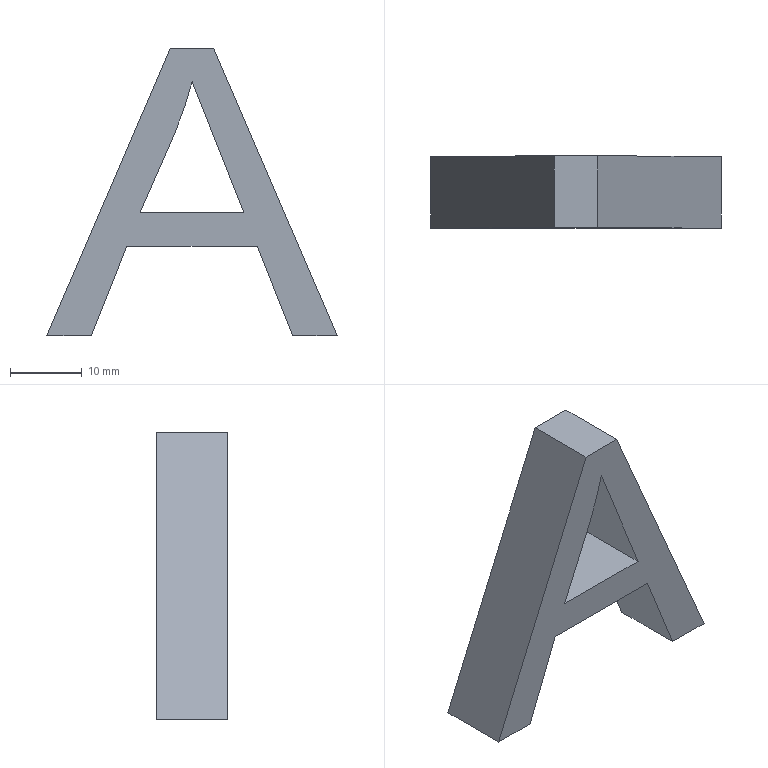Part | NX | features solid 2 | 1 solid | 14 faces | box 40.444 x 10 x 40 mm | volume 5154 mm3 | plane 12 | spline 2
STEP:
#1=CARTESIAN_POINT('',(-526.132,-915.,172.421));
#2=VERTEX_POINT('',#1);
#3=CARTESIAN_POINT('',(-533.352,-915.,190.669));
#4=VERTEX_POINT('',#3);
#5=CARTESIAN_POINT('',(-526.132,-915.,172.421));
#6=CARTESIAN_POINT('',(-527.509,-915.,175.908));
#7=CARTESIAN_POINT('',(-528.886,-915.,179.396));
#8=CARTESIAN_POINT('',(-531.586,-915.,186.236));
#9=CARTESIAN_POINT('',(-532.618,-915.,188.834));
#10=CARTESIAN_POINT('',(-533.352,-915.,190.669));
#11=B_SPLINE_CURVE_WITH_KNOTS('',3,(#5,#6,#7,#8,#9,#10),.UNSPECIFIED.,.F.,.F.,(4,2,4),(0.4694,0.6682,0.8594),.UNSPECIFIED.);
#12=EDGE_CURVE('',#2,#4,#11,.T.);
#13=ORIENTED_EDGE('',*,*,#12,.F.);
#14=CARTESIAN_POINT('',(-526.132,-925.,172.421));
#15=VERTEX_POINT('',#14);
#16=CARTESIAN_POINT('',(-526.132,-925.,172.421));
#17=DIRECTION('',(0.,1.,0.));
#18=VECTOR('',#17,1000.);
#19=LINE('',#16,#18);
#20=EDGE_CURVE('',#15,#2,#19,.T.);
#21=ORIENTED_EDGE('',*,*,#20,.F.);
#22=CARTESIAN_POINT('',(-533.352,-925.,190.669));
#23=VERTEX_POINT('',#22);
#24=CARTESIAN_POINT('',(-526.132,-925.,172.421));
#25=CARTESIAN_POINT('',(-527.509,-925.,175.908));
#26=CARTESIAN_POINT('',(-528.886,-925.,179.396));
#27=CARTESIAN_POINT('',(-531.586,-925.,186.236));
#28=CARTESIAN_POINT('',(-532.618,-925.,188.834));
#29=CARTESIAN_POINT('',(-533.352,-925.,190.669));
#30=B_SPLINE_CURVE_WITH_KNOTS('',3,(#24,#25,#26,#27,#28,#29),.UNSPECIFIED.,.F.,.F.,(4,2,4),(0.4694,0.6682,0.8594),.UNSPECIFIED.);
#31=EDGE_CURVE('',#15,#23,#30,.T.);
#32=ORIENTED_EDGE('',*,*,#31,.T.);
#33=CARTESIAN_POINT('',(-533.352,-925.,190.669));
#34=DIRECTION('',(0.,1.,0.));
#35=VECTOR('',#34,1000.);
#36=LINE('',#33,#35);
#37=EDGE_CURVE('',#23,#4,#36,.T.);
#38=ORIENTED_EDGE('',*,*,#37,.T.);
#39=EDGE_LOOP('',(#13,#21,#32,#38));
#40=FACE_BOUND('',#39,.T.);
#41=CARTESIAN_POINT('',(-526.132,-925.,172.421));
#42=CARTESIAN_POINT('',(-526.132,-915.,172.421));
#43=CARTESIAN_POINT('',(-526.807,-925.,174.131));
#44=CARTESIAN_POINT('',(-526.807,-915.,174.131));
#45=CARTESIAN_POINT('',(-527.821,-925.,176.699));
#46=CARTESIAN_POINT('',(-527.821,-915.,176.699));
#47=CARTESIAN_POINT('',(-529.168,-925.,180.111));
#48=CARTESIAN_POINT('',(-529.168,-915.,180.111));
#49=CARTESIAN_POINT('',(-530.19,-925.,182.699));
#50=CARTESIAN_POINT('',(-530.19,-915.,182.699));
#51=CARTESIAN_POINT('',(-531.169,-925.,185.178));
#52=CARTESIAN_POINT('',(-531.169,-915.,185.178));
#53=CARTESIAN_POINT('',(-532.298,-925.,188.027));
#54=CARTESIAN_POINT('',(-532.298,-915.,188.027));
#55=CARTESIAN_POINT('',(-532.978,-925.,189.733));
#56=CARTESIAN_POINT('',(-532.978,-915.,189.733));
#57=CARTESIAN_POINT('',(-533.352,-925.,190.669));
#58=CARTESIAN_POINT('',(-533.352,-915.,190.669));
#59=B_SPLINE_SURFACE_WITH_KNOTS('',3,1,((#41,#42),(#43,#44),(#45,#46),(#47,#48),(#49,#50),(#51,#52),(#53,#54),(#55,#56),(#57,#58)),.SURF_OF_LINEAR_EXTRUSION.,.F.,.F.,.F.,(4,1,1,1,1,1,4),(2,2),(0.4694,0.5669,0.6156,0.6644,0.7131,0.7619,0.8594),(0.,1.),.UNSPECIFIED.);
#60=ADVANCED_FACE('',(#40),#59,.T.);
#61=CARTESIAN_POINT('',(-535.754,-915.,183.511));
#62=VERTEX_POINT('',#61);
#63=CARTESIAN_POINT('',(-533.352,-915.,190.669));
#64=CARTESIAN_POINT('',(-533.918,-915.,188.39));
#65=CARTESIAN_POINT('',(-534.729,-915.,186.004));
#66=CARTESIAN_POINT('',(-535.754,-915.,183.511));
#67=B_SPLINE_CURVE_WITH_KNOTS('',3,(#63,#64,#65,#66),.UNSPECIFIED.,.F.,.F.,(4,4),(0.8594,1.),.PIECEWISE_BEZIER_KNOTS.);
#68=EDGE_CURVE('',#4,#62,#67,.T.);
#69=ORIENTED_EDGE('',*,*,#68,.F.);
#70=ORIENTED_EDGE('',*,*,#37,.F.);
#71=CARTESIAN_POINT('',(-535.754,-925.,183.511));
#72=VERTEX_POINT('',#71);
#73=CARTESIAN_POINT('',(-533.352,-925.,190.669));
#74=CARTESIAN_POINT('',(-533.918,-925.,188.39));
#75=CARTESIAN_POINT('',(-534.729,-925.,186.004));
#76=CARTESIAN_POINT('',(-535.754,-925.,183.511));
#77=B_SPLINE_CURVE_WITH_KNOTS('',3,(#73,#74,#75,#76),.UNSPECIFIED.,.F.,.F.,(4,4),(0.8594,1.),.PIECEWISE_BEZIER_KNOTS.);
#78=EDGE_CURVE('',#23,#72,#77,.T.);
#79=ORIENTED_EDGE('',*,*,#78,.T.);
#80=CARTESIAN_POINT('',(-535.754,-925.,183.511));
#81=DIRECTION('',(0.,1.,0.));
#82=VECTOR('',#81,1000.);
#83=LINE('',#80,#82);
#84=EDGE_CURVE('',#72,#62,#83,.T.);
#85=ORIENTED_EDGE('',*,*,#84,.T.);
#86=EDGE_LOOP('',(#69,#70,#79,#85));
#87=FACE_BOUND('',#86,.T.);
#88=CARTESIAN_POINT('',(-533.352,-925.,190.669));
#89=CARTESIAN_POINT('',(-533.352,-915.,190.669));
#90=CARTESIAN_POINT('',(-533.918,-925.,188.39));
#91=CARTESIAN_POINT('',(-533.918,-915.,188.39));
#92=CARTESIAN_POINT('',(-534.729,-925.,186.004));
#93=CARTESIAN_POINT('',(-534.729,-915.,186.004));
#94=CARTESIAN_POINT('',(-535.754,-925.,183.511));
#95=CARTESIAN_POINT('',(-535.754,-915.,183.511));
#96=B_SPLINE_SURFACE_WITH_KNOTS('',3,1,((#88,#89),(#90,#91),(#92,#93),(#94,#95)),.SURF_OF_LINEAR_EXTRUSION.,.F.,.F.,.F.,(4,4),(2,2),(0.8594,1.),(0.,1.),.PIECEWISE_BEZIER_KNOTS.);
#97=ADVANCED_FACE('',(#87),#96,.T.);
#98=CARTESIAN_POINT('',(-540.587,-915.,172.421));
#99=VERTEX_POINT('',#98);
#100=CARTESIAN_POINT('',(-535.754,-915.,183.511));
#101=CARTESIAN_POINT('',(-537.365,-915.,179.814));
#102=CARTESIAN_POINT('',(-538.976,-915.,176.117));
#103=CARTESIAN_POINT('',(-540.587,-915.,172.421));
#104=B_SPLINE_CURVE_WITH_KNOTS('',3,(#100,#101,#102,#103),.UNSPECIFIED.,.F.,.F.,(4,4),(0.,0.2138),.PIECEWISE_BEZIER_KNOTS.);
#105=EDGE_CURVE('',#62,#99,#104,.T.);
#106=ORIENTED_EDGE('',*,*,#105,.F.);
#107=ORIENTED_EDGE('',*,*,#84,.F.);
#108=CARTESIAN_POINT('',(-540.587,-925.,172.421));
#109=VERTEX_POINT('',#108);
#110=CARTESIAN_POINT('',(-535.754,-925.,183.511));
#111=CARTESIAN_POINT('',(-537.365,-925.,179.814));
#112=CARTESIAN_POINT('',(-538.976,-925.,176.117));
#113=CARTESIAN_POINT('',(-540.587,-925.,172.421));
#114=B_SPLINE_CURVE_WITH_KNOTS('',3,(#110,#111,#112,#113),.UNSPECIFIED.,.F.,.F.,(4,4),(0.,0.2138),.PIECEWISE_BEZIER_KNOTS.);
#115=EDGE_CURVE('',#72,#109,#114,.T.);
#116=ORIENTED_EDGE('',*,*,#115,.T.);
#117=CARTESIAN_POINT('',(-540.587,-925.,172.421));
#118=DIRECTION('',(0.,1.,0.));
#119=VECTOR('',#118,1000.);
#120=LINE('',#117,#119);
#121=EDGE_CURVE('',#109,#99,#120,.T.);
#122=ORIENTED_EDGE('',*,*,#121,.T.);
#123=EDGE_LOOP('',(#106,#107,#116,#122));
#124=FACE_BOUND('',#123,.T.);
#125=CARTESIAN_POINT('',(-535.754,-925.,183.511));
#126=DIRECTION('',(0.9167,0.,-0.3996));
#127=DIRECTION('',(0.3996,0.,0.9167));
#128=AXIS2_PLACEMENT_3D('',#125,#126,#127);
#129=PLANE('',#128);
#130=ADVANCED_FACE('',(#124),#129,.T.);
#131=CARTESIAN_POINT('',(-547.364,-915.,155.335));
#132=VERTEX_POINT('',#131);
#133=CARTESIAN_POINT('',(-553.574,-915.,155.335));
#134=VERTEX_POINT('',#133);
#135=CARTESIAN_POINT('',(-547.364,-915.,155.335));
#136=CARTESIAN_POINT('',(-549.434,-915.,155.335));
#137=CARTESIAN_POINT('',(-551.504,-915.,155.335));
#138=CARTESIAN_POINT('',(-553.574,-915.,155.335));
#139=B_SPLINE_CURVE_WITH_KNOTS('',3,(#135,#136,#137,#138),.UNSPECIFIED.,.F.,.F.,(4,4),(0.,0.04128),.PIECEWISE_BEZIER_KNOTS.);
#140=EDGE_CURVE('',#132,#134,#139,.T.);
#141=ORIENTED_EDGE('',*,*,#140,.F.);
#142=CARTESIAN_POINT('',(-547.364,-925.,155.335));
#143=VERTEX_POINT('',#142);
#144=CARTESIAN_POINT('',(-547.364,-925.,155.335));
#145=DIRECTION('',(0.,1.,0.));
#146=VECTOR('',#145,1000.);
#147=LINE('',#144,#146);
#148=EDGE_CURVE('',#143,#132,#147,.T.);
#149=ORIENTED_EDGE('',*,*,#148,.F.);
#150=CARTESIAN_POINT('',(-553.574,-925.,155.335));
#151=VERTEX_POINT('',#150);
#152=CARTESIAN_POINT('',(-547.364,-925.,155.335));
#153=CARTESIAN_POINT('',(-549.434,-925.,155.335));
#154=CARTESIAN_POINT('',(-551.504,-925.,155.335));
#155=CARTESIAN_POINT('',(-553.574,-925.,155.335));
#156=B_SPLINE_CURVE_WITH_KNOTS('',3,(#152,#153,#154,#155),.UNSPECIFIED.,.F.,.F.,(4,4),(0.,0.04128),.PIECEWISE_BEZIER_KNOTS.);
#157=EDGE_CURVE('',#143,#151,#156,.T.);
#158=ORIENTED_EDGE('',*,*,#157,.T.);
#159=CARTESIAN_POINT('',(-553.574,-925.,155.335));
#160=DIRECTION('',(0.,1.,0.));
#161=VECTOR('',#160,1000.);
#162=LINE('',#159,#161);
#163=EDGE_CURVE('',#151,#134,#162,.T.);
#164=ORIENTED_EDGE('',*,*,#163,.T.);
#165=EDGE_LOOP('',(#141,#149,#158,#164));
#166=FACE_BOUND('',#165,.T.);
#167=CARTESIAN_POINT('',(-547.364,-925.,155.335));
#168=DIRECTION('',(0.,0.,-1.));
#169=DIRECTION('',(0.,1.,0.));
#170=AXIS2_PLACEMENT_3D('',#167,#168,#169);
#171=PLANE('',#170);
#172=ADVANCED_FACE('',(#166),#171,.T.);
#173=CARTESIAN_POINT('',(-536.381,-915.,195.335));
#174=VERTEX_POINT('',#173);
#175=CARTESIAN_POINT('',(-553.574,-915.,155.335));
#176=CARTESIAN_POINT('',(-547.843,-915.,168.668));
#177=CARTESIAN_POINT('',(-542.112,-915.,182.001));
#178=CARTESIAN_POINT('',(-536.381,-915.,195.335));
#179=B_SPLINE_CURVE_WITH_KNOTS('',3,(#175,#176,#177,#178),.UNSPECIFIED.,.F.,.F.,(4,4),(0.04128,0.3307),.PIECEWISE_BEZIER_KNOTS.);
#180=EDGE_CURVE('',#134,#174,#179,.T.);
#181=ORIENTED_EDGE('',*,*,#180,.F.);
#182=ORIENTED_EDGE('',*,*,#163,.F.);
#183=CARTESIAN_POINT('',(-536.381,-925.,195.335));
#184=VERTEX_POINT('',#183);
#185=CARTESIAN_POINT('',(-553.574,-925.,155.335));
#186=CARTESIAN_POINT('',(-547.843,-925.,168.668));
#187=CARTESIAN_POINT('',(-542.112,-925.,182.001));
#188=CARTESIAN_POINT('',(-536.381,-925.,195.335));
#189=B_SPLINE_CURVE_WITH_KNOTS('',3,(#185,#186,#187,#188),.UNSPECIFIED.,.F.,.F.,(4,4),(0.04128,0.3307),.PIECEWISE_BEZIER_KNOTS.);
#190=EDGE_CURVE('',#151,#184,#189,.T.);
#191=ORIENTED_EDGE('',*,*,#190,.T.);
#192=CARTESIAN_POINT('',(-536.381,-925.,195.335));
#193=DIRECTION('',(0.,1.,0.));
#194=VECTOR('',#193,1000.);
#195=LINE('',#192,#194);
#196=EDGE_CURVE('',#184,#174,#195,.T.);
#197=ORIENTED_EDGE('',*,*,#196,.T.);
#198=EDGE_LOOP('',(#181,#182,#191,#197));
#199=FACE_BOUND('',#198,.T.);
#200=CARTESIAN_POINT('',(-553.574,-925.,155.335));
#201=DIRECTION('',(-0.9187,0.,0.3949));
#202=DIRECTION('',(-0.3949,0.,-0.9187));
#203=AXIS2_PLACEMENT_3D('',#200,#201,#202);
#204=PLANE('',#203);
#205=ADVANCED_FACE('',(#199),#204,.T.);
#206=CARTESIAN_POINT('',(-530.339,-915.,195.335));
#207=VERTEX_POINT('',#206);
#208=CARTESIAN_POINT('',(-536.381,-915.,195.335));
#209=CARTESIAN_POINT('',(-534.367,-915.,195.335));
#210=CARTESIAN_POINT('',(-532.353,-915.,195.335));
#211=CARTESIAN_POINT('',(-530.339,-915.,195.335));
#212=B_SPLINE_CURVE_WITH_KNOTS('',3,(#208,#209,#210,#211),.UNSPECIFIED.,.F.,.F.,(4,4),(0.3307,0.3709),.PIECEWISE_BEZIER_KNOTS.);
#213=EDGE_CURVE('',#174,#207,#212,.T.);
#214=ORIENTED_EDGE('',*,*,#213,.F.);
#215=ORIENTED_EDGE('',*,*,#196,.F.);
#216=CARTESIAN_POINT('',(-530.339,-925.,195.335));
#217=VERTEX_POINT('',#216);
#218=CARTESIAN_POINT('',(-536.381,-925.,195.335));
#219=CARTESIAN_POINT('',(-534.367,-925.,195.335));
#220=CARTESIAN_POINT('',(-532.353,-925.,195.335));
#221=CARTESIAN_POINT('',(-530.339,-925.,195.335));
#222=B_SPLINE_CURVE_WITH_KNOTS('',3,(#218,#219,#220,#221),.UNSPECIFIED.,.F.,.F.,(4,4),(0.3307,0.3709),.PIECEWISE_BEZIER_KNOTS.);
#223=EDGE_CURVE('',#184,#217,#222,.T.);
#224=ORIENTED_EDGE('',*,*,#223,.T.);
#225=CARTESIAN_POINT('',(-530.339,-925.,195.335));
#226=DIRECTION('',(0.,1.,0.));
#227=VECTOR('',#226,1000.);
#228=LINE('',#225,#227);
#229=EDGE_CURVE('',#217,#207,#228,.T.);
#230=ORIENTED_EDGE('',*,*,#229,.T.);
#231=EDGE_LOOP('',(#214,#215,#224,#230));
#232=FACE_BOUND('',#231,.T.);
#233=CARTESIAN_POINT('',(-536.381,-925.,195.335));
#234=DIRECTION('',(0.,0.,1.));
#235=DIRECTION('',(0.,-1.,0.));
#236=AXIS2_PLACEMENT_3D('',#233,#234,#235);
#237=PLANE('',#236);
#238=ADVANCED_FACE('',(#232),#237,.T.);
#239=CARTESIAN_POINT('',(-513.13,-915.,155.335));
#240=VERTEX_POINT('',#239);
#241=CARTESIAN_POINT('',(-530.339,-915.,195.335));
#242=CARTESIAN_POINT('',(-524.603,-915.,182.001));
#243=CARTESIAN_POINT('',(-518.867,-915.,168.668));
#244=CARTESIAN_POINT('',(-513.13,-915.,155.335));
#245=B_SPLINE_CURVE_WITH_KNOTS('',3,(#241,#242,#243,#244),.UNSPECIFIED.,.F.,.F.,(4,4),(0.3709,0.6603),.PIECEWISE_BEZIER_KNOTS.);
#246=EDGE_CURVE('',#207,#240,#245,.T.);
#247=ORIENTED_EDGE('',*,*,#246,.F.);
#248=ORIENTED_EDGE('',*,*,#229,.F.);
#249=CARTESIAN_POINT('',(-513.13,-925.,155.335));
#250=VERTEX_POINT('',#249);
#251=CARTESIAN_POINT('',(-530.339,-925.,195.335));
#252=CARTESIAN_POINT('',(-524.603,-925.,182.001));
#253=CARTESIAN_POINT('',(-518.867,-925.,168.668));
#254=CARTESIAN_POINT('',(-513.13,-925.,155.335));
#255=B_SPLINE_CURVE_WITH_KNOTS('',3,(#251,#252,#253,#254),.UNSPECIFIED.,.F.,.F.,(4,4),(0.3709,0.6603),.PIECEWISE_BEZIER_KNOTS.);
#256=EDGE_CURVE('',#217,#250,#255,.T.);
#257=ORIENTED_EDGE('',*,*,#256,.T.);
#258=CARTESIAN_POINT('',(-513.13,-925.,155.335));
#259=DIRECTION('',(0.,1.,0.));
#260=VECTOR('',#259,1000.);
#261=LINE('',#258,#260);
#262=EDGE_CURVE('',#250,#240,#261,.T.);
#263=ORIENTED_EDGE('',*,*,#262,.T.);
#264=EDGE_LOOP('',(#247,#248,#257,#263));
#265=FACE_BOUND('',#264,.T.);
#266=CARTESIAN_POINT('',(-530.339,-925.,195.335));
#267=DIRECTION('',(0.9186,0.,0.3952));
#268=DIRECTION('',(-0.3952,0.,0.9186));
#269=AXIS2_PLACEMENT_3D('',#266,#267,#268);
#270=PLANE('',#269);
#271=ADVANCED_FACE('',(#265),#270,.T.);
#272=CARTESIAN_POINT('',(-519.325,-915.,155.335));
#273=VERTEX_POINT('',#272);
#274=CARTESIAN_POINT('',(-513.13,-915.,155.335));
#275=CARTESIAN_POINT('',(-515.195,-915.,155.335));
#276=CARTESIAN_POINT('',(-517.26,-915.,155.335));
#277=CARTESIAN_POINT('',(-519.325,-915.,155.335));
#278=B_SPLINE_CURVE_WITH_KNOTS('',3,(#274,#275,#276,#277),.UNSPECIFIED.,.F.,.F.,(4,4),(0.6603,0.7015),.PIECEWISE_BEZIER_KNOTS.);
#279=EDGE_CURVE('',#240,#273,#278,.T.);
#280=ORIENTED_EDGE('',*,*,#279,.F.);
#281=ORIENTED_EDGE('',*,*,#262,.F.);
#282=CARTESIAN_POINT('',(-519.325,-925.,155.335));
#283=VERTEX_POINT('',#282);
#284=CARTESIAN_POINT('',(-513.13,-925.,155.335));
#285=CARTESIAN_POINT('',(-515.195,-925.,155.335));
#286=CARTESIAN_POINT('',(-517.26,-925.,155.335));
#287=CARTESIAN_POINT('',(-519.325,-925.,155.335));
#288=B_SPLINE_CURVE_WITH_KNOTS('',3,(#284,#285,#286,#287),.UNSPECIFIED.,.F.,.F.,(4,4),(0.6603,0.7015),.PIECEWISE_BEZIER_KNOTS.);
#289=EDGE_CURVE('',#250,#283,#288,.T.);
#290=ORIENTED_EDGE('',*,*,#289,.T.);
#291=CARTESIAN_POINT('',(-519.325,-925.,155.335));
#292=DIRECTION('',(0.,1.,0.));
#293=VECTOR('',#292,1000.);
#294=LINE('',#291,#293);
#295=EDGE_CURVE('',#283,#273,#294,.T.);
#296=ORIENTED_EDGE('',*,*,#295,.T.);
#297=EDGE_LOOP('',(#280,#281,#290,#296));
#298=FACE_BOUND('',#297,.T.);
#299=CARTESIAN_POINT('',(-513.13,-925.,155.335));
#300=DIRECTION('',(0.,0.,-1.));
#301=DIRECTION('',(0.,1.,0.));
#302=AXIS2_PLACEMENT_3D('',#299,#300,#301);
#303=PLANE('',#302);
#304=ADVANCED_FACE('',(#298),#303,.T.);
#305=CARTESIAN_POINT('',(-524.266,-915.,167.755));
#306=VERTEX_POINT('',#305);
#307=CARTESIAN_POINT('',(-519.325,-915.,155.335));
#308=CARTESIAN_POINT('',(-520.972,-915.,159.475));
#309=CARTESIAN_POINT('',(-522.619,-915.,163.615));
#310=CARTESIAN_POINT('',(-524.266,-915.,167.755));
#311=B_SPLINE_CURVE_WITH_KNOTS('',3,(#307,#308,#309,#310),.UNSPECIFIED.,.F.,.F.,(4,4),(0.7015,0.7904),.PIECEWISE_BEZIER_KNOTS.);
#312=EDGE_CURVE('',#273,#306,#311,.T.);
#313=ORIENTED_EDGE('',*,*,#312,.F.);
#314=ORIENTED_EDGE('',*,*,#295,.F.);
#315=CARTESIAN_POINT('',(-524.266,-925.,167.755));
#316=VERTEX_POINT('',#315);
#317=CARTESIAN_POINT('',(-519.325,-925.,155.335));
#318=CARTESIAN_POINT('',(-520.972,-925.,159.475));
#319=CARTESIAN_POINT('',(-522.619,-925.,163.615));
#320=CARTESIAN_POINT('',(-524.266,-925.,167.755));
#321=B_SPLINE_CURVE_WITH_KNOTS('',3,(#317,#318,#319,#320),.UNSPECIFIED.,.F.,.F.,(4,4),(0.7015,0.7904),.PIECEWISE_BEZIER_KNOTS.);
#322=EDGE_CURVE('',#283,#316,#321,.T.);
#323=ORIENTED_EDGE('',*,*,#322,.T.);
#324=CARTESIAN_POINT('',(-524.266,-925.,167.755));
#325=DIRECTION('',(0.,1.,0.));
#326=VECTOR('',#325,1000.);
#327=LINE('',#324,#326);
#328=EDGE_CURVE('',#316,#306,#327,.T.);
#329=ORIENTED_EDGE('',*,*,#328,.T.);
#330=EDGE_LOOP('',(#313,#314,#323,#329));
#331=FACE_BOUND('',#330,.T.);
#332=CARTESIAN_POINT('',(-519.325,-925.,155.335));
#333=DIRECTION('',(-0.9292,0.,-0.3696));
#334=DIRECTION('',(0.3696,0.,-0.9292));
#335=AXIS2_PLACEMENT_3D('',#332,#333,#334);
#336=PLANE('',#335);
#337=ADVANCED_FACE('',(#331),#336,.T.);
#338=CARTESIAN_POINT('',(-542.438,-915.,167.755));
#339=VERTEX_POINT('',#338);
#340=CARTESIAN_POINT('',(-524.266,-915.,167.755));
#341=CARTESIAN_POINT('',(-530.324,-915.,167.755));
#342=CARTESIAN_POINT('',(-536.381,-915.,167.755));
#343=CARTESIAN_POINT('',(-542.438,-915.,167.755));
#344=B_SPLINE_CURVE_WITH_KNOTS('',3,(#340,#341,#342,#343),.UNSPECIFIED.,.F.,.F.,(4,4),(0.7904,0.9112),.PIECEWISE_BEZIER_KNOTS.);
#345=EDGE_CURVE('',#306,#339,#344,.T.);
#346=ORIENTED_EDGE('',*,*,#345,.F.);
#347=ORIENTED_EDGE('',*,*,#328,.F.);
#348=CARTESIAN_POINT('',(-542.438,-925.,167.755));
#349=VERTEX_POINT('',#348);
#350=CARTESIAN_POINT('',(-524.266,-925.,167.755));
#351=CARTESIAN_POINT('',(-530.324,-925.,167.755));
#352=CARTESIAN_POINT('',(-536.381,-925.,167.755));
#353=CARTESIAN_POINT('',(-542.438,-925.,167.755));
#354=B_SPLINE_CURVE_WITH_KNOTS('',3,(#350,#351,#352,#353),.UNSPECIFIED.,.F.,.F.,(4,4),(0.7904,0.9112),.PIECEWISE_BEZIER_KNOTS.);
#355=EDGE_CURVE('',#316,#349,#354,.T.);
#356=ORIENTED_EDGE('',*,*,#355,.T.);
#357=CARTESIAN_POINT('',(-542.438,-925.,167.755));
#358=DIRECTION('',(0.,1.,0.));
#359=VECTOR('',#358,1000.);
#360=LINE('',#357,#359);
#361=EDGE_CURVE('',#349,#339,#360,.T.);
#362=ORIENTED_EDGE('',*,*,#361,.T.);
#363=EDGE_LOOP('',(#346,#347,#356,#362));
#364=FACE_BOUND('',#363,.T.);
#365=CARTESIAN_POINT('',(-524.266,-925.,167.755));
#366=DIRECTION('',(0.,0.,-1.));
#367=DIRECTION('',(0.,1.,0.));
#368=AXIS2_PLACEMENT_3D('',#365,#366,#367);
#369=PLANE('',#368);
#370=ADVANCED_FACE('',(#364),#369,.T.);
#371=CARTESIAN_POINT('',(-542.438,-915.,167.755));
#372=CARTESIAN_POINT('',(-544.08,-915.,163.615));
#373=CARTESIAN_POINT('',(-545.722,-915.,159.475));
#374=CARTESIAN_POINT('',(-547.364,-915.,155.335));
#375=B_SPLINE_CURVE_WITH_KNOTS('',3,(#371,#372,#373,#374),.UNSPECIFIED.,.F.,.F.,(4,4),(0.9112,1.),.PIECEWISE_BEZIER_KNOTS.);
#376=EDGE_CURVE('',#339,#132,#375,.T.);
#377=ORIENTED_EDGE('',*,*,#376,.F.);
#378=ORIENTED_EDGE('',*,*,#361,.F.);
#379=CARTESIAN_POINT('',(-542.438,-925.,167.755));
#380=CARTESIAN_POINT('',(-544.08,-925.,163.615));
#381=CARTESIAN_POINT('',(-545.722,-925.,159.475));
#382=CARTESIAN_POINT('',(-547.364,-925.,155.335));
#383=B_SPLINE_CURVE_WITH_KNOTS('',3,(#379,#380,#381,#382),.UNSPECIFIED.,.F.,.F.,(4,4),(0.9112,1.),.PIECEWISE_BEZIER_KNOTS.);
#384=EDGE_CURVE('',#349,#143,#383,.T.);
#385=ORIENTED_EDGE('',*,*,#384,.T.);
#386=ORIENTED_EDGE('',*,*,#148,.T.);
#387=EDGE_LOOP('',(#377,#378,#385,#386));
#388=FACE_BOUND('',#387,.T.);
#389=CARTESIAN_POINT('',(-542.438,-925.,167.755));
#390=DIRECTION('',(0.9296,0.,-0.3686));
#391=DIRECTION('',(0.3686,0.,0.9296));
#392=AXIS2_PLACEMENT_3D('',#389,#390,#391);
#393=PLANE('',#392);
#394=ADVANCED_FACE('',(#388),#393,.T.);
#395=CARTESIAN_POINT('',(-540.587,-915.,172.421));
#396=CARTESIAN_POINT('',(-535.769,-915.,172.421));
#397=CARTESIAN_POINT('',(-530.951,-915.,172.421));
#398=CARTESIAN_POINT('',(-526.132,-915.,172.421));
#399=B_SPLINE_CURVE_WITH_KNOTS('',3,(#395,#396,#397,#398),.UNSPECIFIED.,.F.,.F.,(4,4),(0.2138,0.4694),.PIECEWISE_BEZIER_KNOTS.);
#400=EDGE_CURVE('',#99,#2,#399,.T.);
#401=ORIENTED_EDGE('',*,*,#400,.F.);
#402=ORIENTED_EDGE('',*,*,#121,.F.);
#403=CARTESIAN_POINT('',(-540.587,-925.,172.421));
#404=CARTESIAN_POINT('',(-535.769,-925.,172.421));
#405=CARTESIAN_POINT('',(-530.951,-925.,172.421));
#406=CARTESIAN_POINT('',(-526.132,-925.,172.421));
#407=B_SPLINE_CURVE_WITH_KNOTS('',3,(#403,#404,#405,#406),.UNSPECIFIED.,.F.,.F.,(4,4),(0.2138,0.4694),.PIECEWISE_BEZIER_KNOTS.);
#408=EDGE_CURVE('',#109,#15,#407,.T.);
#409=ORIENTED_EDGE('',*,*,#408,.T.);
#410=ORIENTED_EDGE('',*,*,#20,.T.);
#411=EDGE_LOOP('',(#401,#402,#409,#410));
#412=FACE_BOUND('',#411,.T.);
#413=CARTESIAN_POINT('',(-540.587,-925.,172.421));
#414=DIRECTION('',(0.,0.,1.));
#415=DIRECTION('',(0.,-1.,0.));
#416=AXIS2_PLACEMENT_3D('',#413,#414,#415);
#417=PLANE('',#416);
#418=ADVANCED_FACE('',(#412),#417,.T.);
#419=ORIENTED_EDGE('',*,*,#157,.F.);
#420=ORIENTED_EDGE('',*,*,#384,.F.);
#421=ORIENTED_EDGE('',*,*,#355,.F.);
#422=ORIENTED_EDGE('',*,*,#322,.F.);
#423=ORIENTED_EDGE('',*,*,#289,.F.);
#424=ORIENTED_EDGE('',*,*,#256,.F.);
#425=ORIENTED_EDGE('',*,*,#223,.F.);
#426=ORIENTED_EDGE('',*,*,#190,.F.);
#427=EDGE_LOOP('',(#419,#420,#421,#422,#423,#424,#425,#426));
#428=FACE_BOUND('',#427,.T.);
#429=ORIENTED_EDGE('',*,*,#31,.F.);
#430=ORIENTED_EDGE('',*,*,#408,.F.);
#431=ORIENTED_EDGE('',*,*,#115,.F.);
#432=ORIENTED_EDGE('',*,*,#78,.F.);
#433=EDGE_LOOP('',(#429,#430,#431,#432));
#434=FACE_BOUND('',#433,.T.);
#435=CARTESIAN_POINT('',(-550.469,-925.,155.335));
#436=DIRECTION('',(0.,-1.,0.));
#437=DIRECTION('',(1.,0.,0.));
#438=AXIS2_PLACEMENT_3D('',#435,#436,#437);
#439=PLANE('',#438);
#440=ADVANCED_FACE('',(#428,#434),#439,.T.);
#441=ORIENTED_EDGE('',*,*,#140,.T.);
#442=ORIENTED_EDGE('',*,*,#180,.T.);
#443=ORIENTED_EDGE('',*,*,#213,.T.);
#444=ORIENTED_EDGE('',*,*,#246,.T.);
#445=ORIENTED_EDGE('',*,*,#279,.T.);
#446=ORIENTED_EDGE('',*,*,#312,.T.);
#447=ORIENTED_EDGE('',*,*,#345,.T.);
#448=ORIENTED_EDGE('',*,*,#376,.T.);
#449=EDGE_LOOP('',(#441,#442,#443,#444,#445,#446,#447,#448));
#450=FACE_BOUND('',#449,.T.);
#451=ORIENTED_EDGE('',*,*,#12,.T.);
#452=ORIENTED_EDGE('',*,*,#68,.T.);
#453=ORIENTED_EDGE('',*,*,#105,.T.);
#454=ORIENTED_EDGE('',*,*,#400,.T.);
#455=EDGE_LOOP('',(#451,#452,#453,#454));
#456=FACE_BOUND('',#455,.T.);
#457=CARTESIAN_POINT('',(-550.469,-915.,155.335));
#458=DIRECTION('',(0.,-1.,0.));
#459=DIRECTION('',(1.,0.,0.));
#460=AXIS2_PLACEMENT_3D('',#457,#458,#459);
#461=PLANE('',#460);
#462=ADVANCED_FACE('',(#450,#456),#461,.F.);
#463=CLOSED_SHELL('',(#60,#97,#130,#172,#205,#238,#271,#304,#337,#370,#394,#418,#440,#462));
#464=MANIFOLD_SOLID_BREP('',#463);
#465=(LENGTH_UNIT()NAMED_UNIT(*)SI_UNIT(.MILLI.,.METRE.));
#466=UNCERTAINTY_MEASURE_WITH_UNIT(LENGTH_MEASURE(0.0508),#465,'','');
#467=(NAMED_UNIT(*)PLANE_ANGLE_UNIT()SI_UNIT($,.RADIAN.));
#468=(NAMED_UNIT(*)SI_UNIT($,.STERADIAN.)SOLID_ANGLE_UNIT());
#469=(GEOMETRIC_REPRESENTATION_CONTEXT(3)GLOBAL_UNCERTAINTY_ASSIGNED_CONTEXT((#466))GLOBAL_UNIT_ASSIGNED_CONTEXT((#465,#467,#468))REPRESENTATION_CONTEXT('',''));
#470=ADVANCED_BREP_SHAPE_REPRESENTATION('',(#464),#469);